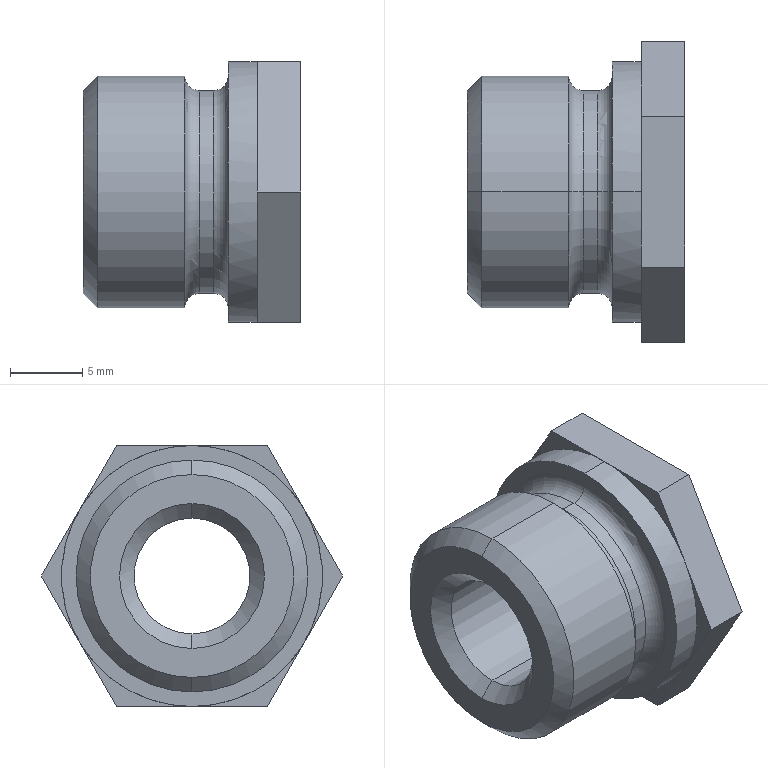Part | SolidWorks | features BaseBody 1 | 1 solid | 33 faces | box 15 x 20.785 x 18 mm | volume 2434 mm3 | plane 15 | cylinder 8 | cone 6 | torus 4 | commonest cylinder face diameters 8 x2 14 x2 16 x2 18 x2
STEP:
#1=CARTESIAN_POINT('',(-9.463,-20.104,-29.75));
#2=VERTEX_POINT('',#1);
#3=CARTESIAN_POINT('',(-9.463,-20.104,-47.75));
#4=VERTEX_POINT('',#3);
#5=CARTESIAN_POINT('',(-9.463,-20.104,-38.75));
#6=DIRECTION('',(-1.,0.,0.));
#7=DIRECTION('',(0.,0.,1.));
#8=AXIS2_PLACEMENT_3D('',#5,#6,#7);
#9=CIRCLE('',#8,9.);
#10=EDGE_CURVE('',#2,#4,#9,.T.);
#11=ORIENTED_EDGE('',*,*,#10,.F.);
#12=CARTESIAN_POINT('',(-7.463,-20.104,-29.75));
#13=VERTEX_POINT('',#12);
#14=CARTESIAN_POINT('',(-9.463,-20.104,-29.75));
#15=DIRECTION('',(1.,0.,0.));
#16=VECTOR('',#15,1000.);
#17=LINE('',#14,#16);
#18=EDGE_CURVE('',#2,#13,#17,.T.);
#19=ORIENTED_EDGE('',*,*,#18,.T.);
#20=CARTESIAN_POINT('',(-7.463,-12.31,-34.25));
#21=VERTEX_POINT('',#20);
#22=CARTESIAN_POINT('',(-7.463,-20.104,-38.75));
#23=DIRECTION('',(-1.,0.,0.));
#24=DIRECTION('',(0.,0.,1.));
#25=AXIS2_PLACEMENT_3D('',#22,#23,#24);
#26=CIRCLE('',#25,9.);
#27=EDGE_CURVE('',#13,#21,#26,.T.);
#28=ORIENTED_EDGE('',*,*,#27,.T.);
#29=CARTESIAN_POINT('',(-7.463,-12.31,-43.25));
#30=VERTEX_POINT('',#29);
#31=CARTESIAN_POINT('',(-7.463,-20.104,-38.75));
#32=DIRECTION('',(-1.,0.,0.));
#33=DIRECTION('',(0.,0.,1.));
#34=AXIS2_PLACEMENT_3D('',#31,#32,#33);
#35=CIRCLE('',#34,9.);
#36=EDGE_CURVE('',#21,#30,#35,.T.);
#37=ORIENTED_EDGE('',*,*,#36,.T.);
#38=CARTESIAN_POINT('',(-7.463,-20.104,-47.75));
#39=VERTEX_POINT('',#38);
#40=CARTESIAN_POINT('',(-7.463,-20.104,-38.75));
#41=DIRECTION('',(-1.,0.,0.));
#42=DIRECTION('',(0.,0.,1.));
#43=AXIS2_PLACEMENT_3D('',#40,#41,#42);
#44=CIRCLE('',#43,9.);
#45=EDGE_CURVE('',#30,#39,#44,.T.);
#46=ORIENTED_EDGE('',*,*,#45,.T.);
#47=CARTESIAN_POINT('',(-9.463,-20.104,-47.75));
#48=DIRECTION('',(1.,0.,0.));
#49=VECTOR('',#48,1000.);
#50=LINE('',#47,#49);
#51=EDGE_CURVE('',#4,#39,#50,.T.);
#52=ORIENTED_EDGE('',*,*,#51,.F.);
#53=EDGE_LOOP('',(#11,#19,#28,#37,#46,#52));
#54=FACE_OUTER_BOUND('',#53,.T.);
#55=CARTESIAN_POINT('',(-9.463,-20.104,-38.75));
#56=DIRECTION('',(1.,0.,0.));
#57=DIRECTION('',(0.,0.,-1.));
#58=AXIS2_PLACEMENT_3D('',#55,#56,#57);
#59=CYLINDRICAL_SURFACE('',#58,9.);
#60=ADVANCED_FACE('',(#54),#59,.T.);
#61=CARTESIAN_POINT('',(-11.463,-20.104,-45.75));
#62=VERTEX_POINT('',#61);
#63=CARTESIAN_POINT('',(-11.463,-20.104,-31.75));
#64=VERTEX_POINT('',#63);
#65=CARTESIAN_POINT('',(-11.463,-20.104,-38.75));
#66=DIRECTION('',(1.,0.,0.));
#67=DIRECTION('',(0.,0.,1.));
#68=AXIS2_PLACEMENT_3D('',#65,#66,#67);
#69=CIRCLE('',#68,7.);
#70=EDGE_CURVE('',#62,#64,#69,.T.);
#71=ORIENTED_EDGE('',*,*,#70,.T.);
#72=CARTESIAN_POINT('',(-10.463,-20.104,-31.75));
#73=VERTEX_POINT('',#72);
#74=CARTESIAN_POINT('',(-12.463,-20.104,-31.75));
#75=DIRECTION('',(1.,0.,0.));
#76=VECTOR('',#75,1000.);
#77=LINE('',#74,#76);
#78=EDGE_CURVE('',#64,#73,#77,.T.);
#79=ORIENTED_EDGE('',*,*,#78,.T.);
#80=CARTESIAN_POINT('',(-10.463,-20.104,-45.75));
#81=VERTEX_POINT('',#80);
#82=CARTESIAN_POINT('',(-10.463,-20.104,-38.75));
#83=DIRECTION('',(-1.,0.,0.));
#84=DIRECTION('',(0.,0.,1.));
#85=AXIS2_PLACEMENT_3D('',#82,#83,#84);
#86=CIRCLE('',#85,7.);
#87=EDGE_CURVE('',#73,#81,#86,.T.);
#88=ORIENTED_EDGE('',*,*,#87,.T.);
#89=CARTESIAN_POINT('',(-12.463,-20.104,-45.75));
#90=DIRECTION('',(1.,0.,0.));
#91=VECTOR('',#90,1000.);
#92=LINE('',#89,#91);
#93=EDGE_CURVE('',#62,#81,#92,.T.);
#94=ORIENTED_EDGE('',*,*,#93,.F.);
#95=EDGE_LOOP('',(#71,#79,#88,#94));
#96=FACE_OUTER_BOUND('',#95,.T.);
#97=CARTESIAN_POINT('',(-12.463,-20.104,-38.75));
#98=DIRECTION('',(1.,0.,0.));
#99=DIRECTION('',(0.,0.,-1.));
#100=AXIS2_PLACEMENT_3D('',#97,#98,#99);
#101=CYLINDRICAL_SURFACE('',#100,7.);
#102=ADVANCED_FACE('',(#96),#101,.T.);
#103=CARTESIAN_POINT('',(-18.463,-20.104,-46.75));
#104=VERTEX_POINT('',#103);
#105=CARTESIAN_POINT('',(-18.463,-20.104,-30.75));
#106=VERTEX_POINT('',#105);
#107=CARTESIAN_POINT('',(-18.463,-20.104,-38.75));
#108=DIRECTION('',(1.,0.,0.));
#109=DIRECTION('',(0.,0.,1.));
#110=AXIS2_PLACEMENT_3D('',#107,#108,#109);
#111=CIRCLE('',#110,8.);
#112=EDGE_CURVE('',#104,#106,#111,.T.);
#113=ORIENTED_EDGE('',*,*,#112,.T.);
#114=CARTESIAN_POINT('',(-12.463,-20.104,-30.75));
#115=VERTEX_POINT('',#114);
#116=CARTESIAN_POINT('',(-19.463,-20.104,-30.75));
#117=DIRECTION('',(1.,0.,0.));
#118=VECTOR('',#117,1000.);
#119=LINE('',#116,#118);
#120=EDGE_CURVE('',#106,#115,#119,.T.);
#121=ORIENTED_EDGE('',*,*,#120,.T.);
#122=CARTESIAN_POINT('',(-12.463,-20.104,-46.75));
#123=VERTEX_POINT('',#122);
#124=CARTESIAN_POINT('',(-12.463,-20.104,-38.75));
#125=DIRECTION('',(-1.,0.,0.));
#126=DIRECTION('',(0.,0.,1.));
#127=AXIS2_PLACEMENT_3D('',#124,#125,#126);
#128=CIRCLE('',#127,8.);
#129=EDGE_CURVE('',#115,#123,#128,.T.);
#130=ORIENTED_EDGE('',*,*,#129,.T.);
#131=CARTESIAN_POINT('',(-19.463,-20.104,-46.75));
#132=DIRECTION('',(1.,0.,0.));
#133=VECTOR('',#132,1000.);
#134=LINE('',#131,#133);
#135=EDGE_CURVE('',#104,#123,#134,.T.);
#136=ORIENTED_EDGE('',*,*,#135,.F.);
#137=EDGE_LOOP('',(#113,#121,#130,#136));
#138=FACE_OUTER_BOUND('',#137,.T.);
#139=CARTESIAN_POINT('',(-19.463,-20.104,-38.75));
#140=DIRECTION('',(1.,0.,0.));
#141=DIRECTION('',(0.,0.,-1.));
#142=AXIS2_PLACEMENT_3D('',#139,#140,#141);
#143=CYLINDRICAL_SURFACE('',#142,8.);
#144=ADVANCED_FACE('',(#138),#143,.T.);
#145=CARTESIAN_POINT('',(-10.463,-20.104,-38.75));
#146=DIRECTION('',(-1.,0.,0.));
#147=DIRECTION('',(0.,0.,1.));
#148=AXIS2_PLACEMENT_3D('',#145,#146,#147);
#149=CIRCLE('',#148,7.);
#150=EDGE_CURVE('',#81,#73,#149,.T.);
#151=ORIENTED_EDGE('',*,*,#150,.F.);
#152=CARTESIAN_POINT('',(-9.463,-20.104,-46.75));
#153=VERTEX_POINT('',#152);
#154=CARTESIAN_POINT('',(-10.463,-20.104,-46.75));
#155=DIRECTION('',(0.,1.,0.));
#156=DIRECTION('',(0.,0.,1.));
#157=AXIS2_PLACEMENT_3D('',#154,#155,#156);
#158=CIRCLE('',#157,1.);
#159=EDGE_CURVE('',#81,#153,#158,.T.);
#160=ORIENTED_EDGE('',*,*,#159,.T.);
#161=CARTESIAN_POINT('',(-9.463,-20.104,-30.75));
#162=VERTEX_POINT('',#161);
#163=CARTESIAN_POINT('',(-9.463,-20.104,-38.75));
#164=DIRECTION('',(1.,0.,0.));
#165=DIRECTION('',(0.,0.,1.));
#166=AXIS2_PLACEMENT_3D('',#163,#164,#165);
#167=CIRCLE('',#166,8.);
#168=EDGE_CURVE('',#162,#153,#167,.T.);
#169=ORIENTED_EDGE('',*,*,#168,.F.);
#170=CARTESIAN_POINT('',(-10.463,-20.104,-30.75));
#171=DIRECTION('',(0.,-1.,0.));
#172=DIRECTION('',(0.,0.,-1.));
#173=AXIS2_PLACEMENT_3D('',#170,#171,#172);
#174=CIRCLE('',#173,1.);
#175=EDGE_CURVE('',#73,#162,#174,.T.);
#176=ORIENTED_EDGE('',*,*,#175,.F.);
#177=EDGE_LOOP('',(#151,#160,#169,#176));
#178=FACE_OUTER_BOUND('',#177,.T.);
#179=CARTESIAN_POINT('',(-10.463,-20.104,-38.75));
#180=DIRECTION('',(-1.,0.,0.));
#181=DIRECTION('',(0.,0.,1.));
#182=AXIS2_PLACEMENT_3D('',#179,#180,#181);
#183=TOROIDAL_SURFACE('',#182,8.,1.);
#184=ADVANCED_FACE('',(#178),#183,.F.);
#185=CARTESIAN_POINT('',(-12.463,-20.104,-38.75));
#186=DIRECTION('',(-1.,0.,0.));
#187=DIRECTION('',(0.,0.,1.));
#188=AXIS2_PLACEMENT_3D('',#185,#186,#187);
#189=CIRCLE('',#188,8.);
#190=EDGE_CURVE('',#123,#115,#189,.T.);
#191=ORIENTED_EDGE('',*,*,#190,.F.);
#192=CARTESIAN_POINT('',(-11.463,-20.104,-46.75));
#193=DIRECTION('',(0.,1.,0.));
#194=DIRECTION('',(0.,0.,1.));
#195=AXIS2_PLACEMENT_3D('',#192,#193,#194);
#196=CIRCLE('',#195,1.);
#197=EDGE_CURVE('',#123,#62,#196,.T.);
#198=ORIENTED_EDGE('',*,*,#197,.T.);
#199=CARTESIAN_POINT('',(-11.463,-20.104,-38.75));
#200=DIRECTION('',(1.,0.,0.));
#201=DIRECTION('',(0.,0.,1.));
#202=AXIS2_PLACEMENT_3D('',#199,#200,#201);
#203=CIRCLE('',#202,7.);
#204=EDGE_CURVE('',#64,#62,#203,.T.);
#205=ORIENTED_EDGE('',*,*,#204,.F.);
#206=CARTESIAN_POINT('',(-11.463,-20.104,-30.75));
#207=DIRECTION('',(0.,-1.,0.));
#208=DIRECTION('',(0.,0.,-1.));
#209=AXIS2_PLACEMENT_3D('',#206,#207,#208);
#210=CIRCLE('',#209,1.);
#211=EDGE_CURVE('',#115,#64,#210,.T.);
#212=ORIENTED_EDGE('',*,*,#211,.F.);
#213=EDGE_LOOP('',(#191,#198,#205,#212));
#214=FACE_OUTER_BOUND('',#213,.T.);
#215=CARTESIAN_POINT('',(-11.463,-20.104,-38.75));
#216=DIRECTION('',(-1.,0.,0.));
#217=DIRECTION('',(0.,0.,1.));
#218=AXIS2_PLACEMENT_3D('',#215,#216,#217);
#219=TOROIDAL_SURFACE('',#218,8.,1.);
#220=ADVANCED_FACE('',(#214),#219,.F.);
#221=CARTESIAN_POINT('',(-19.463,-20.104,-31.75));
#222=VERTEX_POINT('',#221);
#223=CARTESIAN_POINT('',(-19.463,-20.104,-45.75));
#224=VERTEX_POINT('',#223);
#225=CARTESIAN_POINT('',(-19.463,-20.104,-38.75));
#226=DIRECTION('',(-1.,0.,0.));
#227=DIRECTION('',(0.,0.,1.));
#228=AXIS2_PLACEMENT_3D('',#225,#226,#227);
#229=CIRCLE('',#228,7.);
#230=EDGE_CURVE('',#222,#224,#229,.T.);
#231=ORIENTED_EDGE('',*,*,#230,.F.);
#232=CARTESIAN_POINT('',(-19.463,-20.104,-31.75));
#233=DIRECTION('',(0.7071,0.,0.7071));
#234=VECTOR('',#233,1000.);
#235=LINE('',#232,#234);
#236=EDGE_CURVE('',#222,#106,#235,.T.);
#237=ORIENTED_EDGE('',*,*,#236,.T.);
#238=ORIENTED_EDGE('',*,*,#112,.F.);
#239=CARTESIAN_POINT('',(-19.463,-20.104,-45.75));
#240=DIRECTION('',(0.7071,0.,-0.7071));
#241=VECTOR('',#240,1000.);
#242=LINE('',#239,#241);
#243=EDGE_CURVE('',#224,#104,#242,.T.);
#244=ORIENTED_EDGE('',*,*,#243,.F.);
#245=EDGE_LOOP('',(#231,#237,#238,#244));
#246=FACE_OUTER_BOUND('',#245,.T.);
#247=CARTESIAN_POINT('',(-19.463,-20.104,-38.75));
#248=DIRECTION('',(1.,0.,0.));
#249=DIRECTION('',(0.,0.,-1.));
#250=AXIS2_PLACEMENT_3D('',#247,#248,#249);
#251=CONICAL_SURFACE('',#250,7.,0.7854);
#252=ADVANCED_FACE('',(#246),#251,.T.);
#253=CARTESIAN_POINT('',(-5.463,-20.104,-34.75));
#254=VERTEX_POINT('',#253);
#255=CARTESIAN_POINT('',(-5.463,-20.104,-42.75));
#256=VERTEX_POINT('',#255);
#257=CARTESIAN_POINT('',(-5.463,-20.104,-38.75));
#258=DIRECTION('',(1.,0.,0.));
#259=DIRECTION('',(0.,0.,1.));
#260=AXIS2_PLACEMENT_3D('',#257,#258,#259);
#261=CIRCLE('',#260,4.);
#262=EDGE_CURVE('',#254,#256,#261,.T.);
#263=ORIENTED_EDGE('',*,*,#262,.T.);
#264=CARTESIAN_POINT('',(-18.463,-20.104,-42.75));
#265=VERTEX_POINT('',#264);
#266=CARTESIAN_POINT('',(-4.463,-20.104,-42.75));
#267=DIRECTION('',(-1.,0.,0.));
#268=VECTOR('',#267,1000.);
#269=LINE('',#266,#268);
#270=EDGE_CURVE('',#256,#265,#269,.T.);
#271=ORIENTED_EDGE('',*,*,#270,.T.);
#272=CARTESIAN_POINT('',(-18.463,-20.104,-34.75));
#273=VERTEX_POINT('',#272);
#274=CARTESIAN_POINT('',(-18.463,-20.104,-38.75));
#275=DIRECTION('',(-1.,0.,0.));
#276=DIRECTION('',(0.,0.,1.));
#277=AXIS2_PLACEMENT_3D('',#274,#275,#276);
#278=CIRCLE('',#277,4.);
#279=EDGE_CURVE('',#265,#273,#278,.T.);
#280=ORIENTED_EDGE('',*,*,#279,.T.);
#281=CARTESIAN_POINT('',(-4.463,-20.104,-34.75));
#282=DIRECTION('',(-1.,0.,0.));
#283=VECTOR('',#282,1000.);
#284=LINE('',#281,#283);
#285=EDGE_CURVE('',#254,#273,#284,.T.);
#286=ORIENTED_EDGE('',*,*,#285,.F.);
#287=EDGE_LOOP('',(#263,#271,#280,#286));
#288=FACE_OUTER_BOUND('',#287,.T.);
#289=CARTESIAN_POINT('',(-4.463,-20.104,-38.75));
#290=DIRECTION('',(-1.,0.,0.));
#291=DIRECTION('',(0.,0.,1.));
#292=AXIS2_PLACEMENT_3D('',#289,#290,#291);
#293=CYLINDRICAL_SURFACE('',#292,4.);
#294=ADVANCED_FACE('',(#288),#293,.F.);
#295=ORIENTED_EDGE('',*,*,#279,.F.);
#296=CARTESIAN_POINT('',(-19.463,-20.104,-43.75));
#297=VERTEX_POINT('',#296);
#298=CARTESIAN_POINT('',(-18.463,-20.104,-42.75));
#299=DIRECTION('',(-0.7071,0.,-0.7071));
#300=VECTOR('',#299,1000.);
#301=LINE('',#298,#300);
#302=EDGE_CURVE('',#265,#297,#301,.T.);
#303=ORIENTED_EDGE('',*,*,#302,.T.);
#304=CARTESIAN_POINT('',(-19.463,-20.104,-33.75));
#305=VERTEX_POINT('',#304);
#306=CARTESIAN_POINT('',(-19.463,-20.104,-38.75));
#307=DIRECTION('',(1.,0.,0.));
#308=DIRECTION('',(0.,0.,1.));
#309=AXIS2_PLACEMENT_3D('',#306,#307,#308);
#310=CIRCLE('',#309,5.);
#311=EDGE_CURVE('',#305,#297,#310,.T.);
#312=ORIENTED_EDGE('',*,*,#311,.F.);
#313=CARTESIAN_POINT('',(-18.463,-20.104,-34.75));
#314=DIRECTION('',(-0.7071,0.,0.7071));
#315=VECTOR('',#314,1000.);
#316=LINE('',#313,#315);
#317=EDGE_CURVE('',#273,#305,#316,.T.);
#318=ORIENTED_EDGE('',*,*,#317,.F.);
#319=EDGE_LOOP('',(#295,#303,#312,#318));
#320=FACE_OUTER_BOUND('',#319,.T.);
#321=CARTESIAN_POINT('',(-18.463,-20.104,-38.75));
#322=DIRECTION('',(-1.,0.,0.));
#323=DIRECTION('',(0.,0.,1.));
#324=AXIS2_PLACEMENT_3D('',#321,#322,#323);
#325=CONICAL_SURFACE('',#324,4.,0.7854);
#326=ADVANCED_FACE('',(#320),#325,.F.);
#327=ORIENTED_EDGE('',*,*,#262,.F.);
#328=CARTESIAN_POINT('',(-4.463,-20.104,-33.75));
#329=VERTEX_POINT('',#328);
#330=CARTESIAN_POINT('',(-4.463,-20.104,-33.75));
#331=DIRECTION('',(0.7071,0.,0.7071));
#332=VECTOR('',#331,1000.);
#333=LINE('',#330,#332);
#334=EDGE_CURVE('',#254,#329,#333,.T.);
#335=ORIENTED_EDGE('',*,*,#334,.T.);
#336=CARTESIAN_POINT('',(-4.463,-20.104,-43.75));
#337=VERTEX_POINT('',#336);
#338=CARTESIAN_POINT('',(-4.463,-20.104,-38.75));
#339=DIRECTION('',(-1.,0.,0.));
#340=DIRECTION('',(0.,0.,1.));
#341=AXIS2_PLACEMENT_3D('',#338,#339,#340);
#342=CIRCLE('',#341,5.);
#343=EDGE_CURVE('',#337,#329,#342,.T.);
#344=ORIENTED_EDGE('',*,*,#343,.F.);
#345=CARTESIAN_POINT('',(-4.463,-20.104,-43.75));
#346=DIRECTION('',(0.7071,0.,-0.7071));
#347=VECTOR('',#346,1000.);
#348=LINE('',#345,#347);
#349=EDGE_CURVE('',#256,#337,#348,.T.);
#350=ORIENTED_EDGE('',*,*,#349,.F.);
#351=EDGE_LOOP('',(#327,#335,#344,#350));
#352=FACE_OUTER_BOUND('',#351,.T.);
#353=CARTESIAN_POINT('',(-4.463,-20.104,-38.75));
#354=DIRECTION('',(1.,0.,0.));
#355=DIRECTION('',(0.,0.,-1.));
#356=AXIS2_PLACEMENT_3D('',#353,#354,#355);
#357=CONICAL_SURFACE('',#356,5.,0.7854);
#358=ADVANCED_FACE('',(#352),#357,.F.);
#359=ORIENTED_EDGE('',*,*,#334,.F.);
#360=CARTESIAN_POINT('',(-5.463,-20.104,-38.75));
#361=DIRECTION('',(1.,0.,0.));
#362=DIRECTION('',(0.,0.,1.));
#363=AXIS2_PLACEMENT_3D('',#360,#361,#362);
#364=CIRCLE('',#363,4.);
#365=EDGE_CURVE('',#256,#254,#364,.T.);
#366=ORIENTED_EDGE('',*,*,#365,.F.);
#367=ORIENTED_EDGE('',*,*,#349,.T.);
#368=CARTESIAN_POINT('',(-4.463,-20.104,-38.75));
#369=DIRECTION('',(-1.,0.,0.));
#370=DIRECTION('',(0.,0.,1.));
#371=AXIS2_PLACEMENT_3D('',#368,#369,#370);
#372=CIRCLE('',#371,5.);
#373=EDGE_CURVE('',#329,#337,#372,.T.);
#374=ORIENTED_EDGE('',*,*,#373,.F.);
#375=EDGE_LOOP('',(#359,#366,#367,#374));
#376=FACE_OUTER_BOUND('',#375,.T.);
#377=CARTESIAN_POINT('',(-4.463,-20.104,-38.75));
#378=DIRECTION('',(1.,0.,0.));
#379=DIRECTION('',(0.,0.,-1.));
#380=AXIS2_PLACEMENT_3D('',#377,#378,#379);
#381=CONICAL_SURFACE('',#380,5.,0.7854);
#382=ADVANCED_FACE('',(#376),#381,.F.);
#383=ORIENTED_EDGE('',*,*,#302,.F.);
#384=CARTESIAN_POINT('',(-18.463,-20.104,-38.75));
#385=DIRECTION('',(-1.,0.,0.));
#386=DIRECTION('',(0.,0.,1.));
#387=AXIS2_PLACEMENT_3D('',#384,#385,#386);
#388=CIRCLE('',#387,4.);
#389=EDGE_CURVE('',#273,#265,#388,.T.);
#390=ORIENTED_EDGE('',*,*,#389,.F.);
#391=ORIENTED_EDGE('',*,*,#317,.T.);
#392=CARTESIAN_POINT('',(-19.463,-20.104,-38.75));
#393=DIRECTION('',(1.,0.,0.));
#394=DIRECTION('',(0.,0.,1.));
#395=AXIS2_PLACEMENT_3D('',#392,#393,#394);
#396=CIRCLE('',#395,5.);
#397=EDGE_CURVE('',#297,#305,#396,.T.);
#398=ORIENTED_EDGE('',*,*,#397,.F.);
#399=EDGE_LOOP('',(#383,#390,#391,#398));
#400=FACE_OUTER_BOUND('',#399,.T.);
#401=CARTESIAN_POINT('',(-18.463,-20.104,-38.75));
#402=DIRECTION('',(-1.,0.,0.));
#403=DIRECTION('',(0.,0.,1.));
#404=AXIS2_PLACEMENT_3D('',#401,#402,#403);
#405=CONICAL_SURFACE('',#404,4.,0.7854);
#406=ADVANCED_FACE('',(#400),#405,.F.);
#407=ORIENTED_EDGE('',*,*,#270,.F.);
#408=ORIENTED_EDGE('',*,*,#365,.T.);
#409=ORIENTED_EDGE('',*,*,#285,.T.);
#410=ORIENTED_EDGE('',*,*,#389,.T.);
#411=EDGE_LOOP('',(#407,#408,#409,#410));
#412=FACE_OUTER_BOUND('',#411,.T.);
#413=CARTESIAN_POINT('',(-4.463,-20.104,-38.75));
#414=DIRECTION('',(-1.,0.,0.));
#415=DIRECTION('',(0.,0.,1.));
#416=AXIS2_PLACEMENT_3D('',#413,#414,#415);
#417=CYLINDRICAL_SURFACE('',#416,4.);
#418=ADVANCED_FACE('',(#412),#417,.F.);
#419=ORIENTED_EDGE('',*,*,#236,.F.);
#420=CARTESIAN_POINT('',(-19.463,-20.104,-38.75));
#421=DIRECTION('',(-1.,0.,0.));
#422=DIRECTION('',(0.,0.,1.));
#423=AXIS2_PLACEMENT_3D('',#420,#421,#422);
#424=CIRCLE('',#423,7.);
#425=EDGE_CURVE('',#224,#222,#424,.T.);
#426=ORIENTED_EDGE('',*,*,#425,.F.);
#427=ORIENTED_EDGE('',*,*,#243,.T.);
#428=CARTESIAN_POINT('',(-18.463,-20.104,-38.75));
#429=DIRECTION('',(1.,0.,0.));
#430=DIRECTION('',(0.,0.,1.));
#431=AXIS2_PLACEMENT_3D('',#428,#429,#430);
#432=CIRCLE('',#431,8.);
#433=EDGE_CURVE('',#106,#104,#432,.T.);
#434=ORIENTED_EDGE('',*,*,#433,.F.);
#435=EDGE_LOOP('',(#419,#426,#427,#434));
#436=FACE_OUTER_BOUND('',#435,.T.);
#437=CARTESIAN_POINT('',(-19.463,-20.104,-38.75));
#438=DIRECTION('',(1.,0.,0.));
#439=DIRECTION('',(0.,0.,-1.));
#440=AXIS2_PLACEMENT_3D('',#437,#438,#439);
#441=CONICAL_SURFACE('',#440,7.,0.7854);
#442=ADVANCED_FACE('',(#436),#441,.T.);
#443=ORIENTED_EDGE('',*,*,#197,.F.);
#444=ORIENTED_EDGE('',*,*,#129,.F.);
#445=ORIENTED_EDGE('',*,*,#211,.T.);
#446=ORIENTED_EDGE('',*,*,#70,.F.);
#447=EDGE_LOOP('',(#443,#444,#445,#446));
#448=FACE_OUTER_BOUND('',#447,.T.);
#449=CARTESIAN_POINT('',(-11.463,-20.104,-38.75));
#450=DIRECTION('',(-1.,0.,0.));
#451=DIRECTION('',(0.,0.,1.));
#452=AXIS2_PLACEMENT_3D('',#449,#450,#451);
#453=TOROIDAL_SURFACE('',#452,8.,1.);
#454=ADVANCED_FACE('',(#448),#453,.F.);
#455=ORIENTED_EDGE('',*,*,#159,.F.);
#456=ORIENTED_EDGE('',*,*,#87,.F.);
#457=ORIENTED_EDGE('',*,*,#175,.T.);
#458=CARTESIAN_POINT('',(-9.463,-20.104,-38.75));
#459=DIRECTION('',(1.,0.,0.));
#460=DIRECTION('',(0.,0.,1.));
#461=AXIS2_PLACEMENT_3D('',#458,#459,#460);
#462=CIRCLE('',#461,8.);
#463=EDGE_CURVE('',#153,#162,#462,.T.);
#464=ORIENTED_EDGE('',*,*,#463,.F.);
#465=EDGE_LOOP('',(#455,#456,#457,#464));
#466=FACE_OUTER_BOUND('',#465,.T.);
#467=CARTESIAN_POINT('',(-10.463,-20.104,-38.75));
#468=DIRECTION('',(-1.,0.,0.));
#469=DIRECTION('',(0.,0.,1.));
#470=AXIS2_PLACEMENT_3D('',#467,#468,#469);
#471=TOROIDAL_SURFACE('',#470,8.,1.);
#472=ADVANCED_FACE('',(#466),#471,.F.);
#473=ORIENTED_EDGE('',*,*,#425,.T.);
#474=ORIENTED_EDGE('',*,*,#230,.T.);
#475=EDGE_LOOP('',(#473,#474));
#476=FACE_OUTER_BOUND('',#475,.T.);
#477=ORIENTED_EDGE('',*,*,#311,.T.);
#478=ORIENTED_EDGE('',*,*,#397,.T.);
#479=EDGE_LOOP('',(#477,#478));
#480=FACE_BOUND('',#479,.T.);
#481=CARTESIAN_POINT('',(-19.463,-20.104,-38.75));
#482=DIRECTION('',(-1.,0.,0.));
#483=DIRECTION('',(0.,1.,0.));
#484=AXIS2_PLACEMENT_3D('',#481,#482,#483);
#485=PLANE('',#484);
#486=ADVANCED_FACE('',(#476,#480),#485,.T.);
#487=ORIENTED_EDGE('',*,*,#120,.F.);
#488=ORIENTED_EDGE('',*,*,#433,.T.);
#489=ORIENTED_EDGE('',*,*,#135,.T.);
#490=ORIENTED_EDGE('',*,*,#190,.T.);
#491=EDGE_LOOP('',(#487,#488,#489,#490));
#492=FACE_OUTER_BOUND('',#491,.T.);
#493=CARTESIAN_POINT('',(-19.463,-20.104,-38.75));
#494=DIRECTION('',(1.,0.,0.));
#495=DIRECTION('',(0.,0.,-1.));
#496=AXIS2_PLACEMENT_3D('',#493,#494,#495);
#497=CYLINDRICAL_SURFACE('',#496,8.);
#498=ADVANCED_FACE('',(#492),#497,.T.);
#499=ORIENTED_EDGE('',*,*,#78,.F.);
#500=ORIENTED_EDGE('',*,*,#204,.T.);
#501=ORIENTED_EDGE('',*,*,#93,.T.);
#502=ORIENTED_EDGE('',*,*,#150,.T.);
#503=EDGE_LOOP('',(#499,#500,#501,#502));
#504=FACE_OUTER_BOUND('',#503,.T.);
#505=CARTESIAN_POINT('',(-12.463,-20.104,-38.75));
#506=DIRECTION('',(1.,0.,0.));
#507=DIRECTION('',(0.,0.,-1.));
#508=AXIS2_PLACEMENT_3D('',#505,#506,#507);
#509=CYLINDRICAL_SURFACE('',#508,7.);
#510=ADVANCED_FACE('',(#504),#509,.T.);
#511=ORIENTED_EDGE('',*,*,#18,.F.);
#512=CARTESIAN_POINT('',(-9.463,-20.104,-38.75));
#513=DIRECTION('',(-1.,0.,0.));
#514=DIRECTION('',(0.,0.,1.));
#515=AXIS2_PLACEMENT_3D('',#512,#513,#514);
#516=CIRCLE('',#515,9.);
#517=EDGE_CURVE('',#4,#2,#516,.T.);
#518=ORIENTED_EDGE('',*,*,#517,.F.);
#519=ORIENTED_EDGE('',*,*,#51,.T.);
#520=CARTESIAN_POINT('',(-7.463,-27.898,-43.25));
#521=VERTEX_POINT('',#520);
#522=CARTESIAN_POINT('',(-7.463,-20.104,-38.75));
#523=DIRECTION('',(-1.,0.,0.));
#524=DIRECTION('',(0.,0.,1.));
#525=AXIS2_PLACEMENT_3D('',#522,#523,#524);
#526=CIRCLE('',#525,9.);
#527=EDGE_CURVE('',#39,#521,#526,.T.);
#528=ORIENTED_EDGE('',*,*,#527,.T.);
#529=CARTESIAN_POINT('',(-7.463,-27.898,-34.25));
#530=VERTEX_POINT('',#529);
#531=CARTESIAN_POINT('',(-7.463,-20.104,-38.75));
#532=DIRECTION('',(-1.,0.,0.));
#533=DIRECTION('',(0.,0.,1.));
#534=AXIS2_PLACEMENT_3D('',#531,#532,#533);
#535=CIRCLE('',#534,9.);
#536=EDGE_CURVE('',#521,#530,#535,.T.);
#537=ORIENTED_EDGE('',*,*,#536,.T.);
#538=CARTESIAN_POINT('',(-7.463,-20.104,-38.75));
#539=DIRECTION('',(-1.,0.,0.));
#540=DIRECTION('',(0.,0.,1.));
#541=AXIS2_PLACEMENT_3D('',#538,#539,#540);
#542=CIRCLE('',#541,9.);
#543=EDGE_CURVE('',#530,#13,#542,.T.);
#544=ORIENTED_EDGE('',*,*,#543,.T.);
#545=EDGE_LOOP('',(#511,#518,#519,#528,#537,#544));
#546=FACE_OUTER_BOUND('',#545,.T.);
#547=CARTESIAN_POINT('',(-9.463,-20.104,-38.75));
#548=DIRECTION('',(1.,0.,0.));
#549=DIRECTION('',(0.,0.,-1.));
#550=AXIS2_PLACEMENT_3D('',#547,#548,#549);
#551=CYLINDRICAL_SURFACE('',#550,9.);
#552=ADVANCED_FACE('',(#546),#551,.T.);
#553=CARTESIAN_POINT('',(-4.463,-9.711,-38.75));
#554=VERTEX_POINT('',#553);
#555=CARTESIAN_POINT('',(-4.463,-14.908,-47.75));
#556=VERTEX_POINT('',#555);
#557=CARTESIAN_POINT('',(-4.463,-9.711,-38.75));
#558=DIRECTION('',(0.,-0.5,-0.866));
#559=VECTOR('',#558,1000.);
#560=LINE('',#557,#559);
#561=EDGE_CURVE('',#554,#556,#560,.T.);
#562=ORIENTED_EDGE('',*,*,#561,.F.);
#563=CARTESIAN_POINT('',(-4.463,-14.908,-29.75));
#564=VERTEX_POINT('',#563);
#565=CARTESIAN_POINT('',(-4.463,-9.711,-38.75));
#566=DIRECTION('',(0.,0.5,-0.866));
#567=VECTOR('',#566,1000.);
#568=LINE('',#565,#567);
#569=EDGE_CURVE('',#564,#554,#568,.T.);
#570=ORIENTED_EDGE('',*,*,#569,.F.);
#571=CARTESIAN_POINT('',(-4.463,-25.3,-29.75));
#572=VERTEX_POINT('',#571);
#573=CARTESIAN_POINT('',(-4.463,-14.908,-29.75));
#574=DIRECTION('',(0.,1.,0.));
#575=VECTOR('',#574,1000.);
#576=LINE('',#573,#575);
#577=EDGE_CURVE('',#572,#564,#576,.T.);
#578=ORIENTED_EDGE('',*,*,#577,.F.);
#579=CARTESIAN_POINT('',(-4.463,-30.496,-38.75));
#580=VERTEX_POINT('',#579);
#581=CARTESIAN_POINT('',(-4.463,-25.3,-29.75));
#582=DIRECTION('',(0.,0.5,0.866));
#583=VECTOR('',#582,1000.);
#584=LINE('',#581,#583);
#585=EDGE_CURVE('',#580,#572,#584,.T.);
#586=ORIENTED_EDGE('',*,*,#585,.F.);
#587=CARTESIAN_POINT('',(-4.463,-25.3,-47.75));
#588=VERTEX_POINT('',#587);
#589=CARTESIAN_POINT('',(-4.463,-25.3,-47.75));
#590=DIRECTION('',(0.,-0.5,0.866));
#591=VECTOR('',#590,1000.);
#592=LINE('',#589,#591);
#593=EDGE_CURVE('',#588,#580,#592,.T.);
#594=ORIENTED_EDGE('',*,*,#593,.F.);
#595=CARTESIAN_POINT('',(-4.463,-14.908,-47.75));
#596=DIRECTION('',(0.,-1.,0.));
#597=VECTOR('',#596,1000.);
#598=LINE('',#595,#597);
#599=EDGE_CURVE('',#556,#588,#598,.T.);
#600=ORIENTED_EDGE('',*,*,#599,.F.);
#601=EDGE_LOOP('',(#562,#570,#578,#586,#594,#600));
#602=FACE_OUTER_BOUND('',#601,.T.);
#603=ORIENTED_EDGE('',*,*,#343,.T.);
#604=ORIENTED_EDGE('',*,*,#373,.T.);
#605=EDGE_LOOP('',(#603,#604));
#606=FACE_BOUND('',#605,.T.);
#607=CARTESIAN_POINT('',(-4.463,-20.104,-56.75));
#608=DIRECTION('',(-1.,0.,0.));
#609=DIRECTION('',(0.,1.,0.));
#610=AXIS2_PLACEMENT_3D('',#607,#608,#609);
#611=PLANE('',#610);
#612=ADVANCED_FACE('',(#602,#606),#611,.F.);
#613=ORIENTED_EDGE('',*,*,#543,.F.);
#614=CARTESIAN_POINT('',(-7.463,-25.3,-29.75));
#615=VERTEX_POINT('',#614);
#616=CARTESIAN_POINT('',(-7.463,-25.3,-29.75));
#617=DIRECTION('',(0.,0.5,0.866));
#618=VECTOR('',#617,1000.);
#619=LINE('',#616,#618);
#620=EDGE_CURVE('',#530,#615,#619,.T.);
#621=ORIENTED_EDGE('',*,*,#620,.T.);
#622=CARTESIAN_POINT('',(-7.463,-14.908,-29.75));
#623=DIRECTION('',(0.,1.,0.));
#624=VECTOR('',#623,1000.);
#625=LINE('',#622,#624);
#626=EDGE_CURVE('',#615,#13,#625,.T.);
#627=ORIENTED_EDGE('',*,*,#626,.T.);
#628=EDGE_LOOP('',(#613,#621,#627));
#629=FACE_OUTER_BOUND('',#628,.T.);
#630=CARTESIAN_POINT('',(-7.463,-20.104,-56.75));
#631=DIRECTION('',(-1.,0.,0.));
#632=DIRECTION('',(0.,1.,0.));
#633=AXIS2_PLACEMENT_3D('',#630,#631,#632);
#634=PLANE('',#633);
#635=ADVANCED_FACE('',(#629),#634,.T.);
#636=ORIENTED_EDGE('',*,*,#569,.T.);
#637=CARTESIAN_POINT('',(-7.463,-9.711,-38.75));
#638=VERTEX_POINT('',#637);
#639=CARTESIAN_POINT('',(-7.463,-9.711,-38.75));
#640=DIRECTION('',(1.,0.,0.));
#641=VECTOR('',#640,1000.);
#642=LINE('',#639,#641);
#643=EDGE_CURVE('',#638,#554,#642,.T.);
#644=ORIENTED_EDGE('',*,*,#643,.F.);
#645=CARTESIAN_POINT('',(-7.463,-9.711,-38.75));
#646=DIRECTION('',(0.,0.5,-0.866));
#647=VECTOR('',#646,1000.);
#648=LINE('',#645,#647);
#649=EDGE_CURVE('',#21,#638,#648,.T.);
#650=ORIENTED_EDGE('',*,*,#649,.F.);
#651=CARTESIAN_POINT('',(-7.463,-14.908,-29.75));
#652=VERTEX_POINT('',#651);
#653=CARTESIAN_POINT('',(-7.463,-9.711,-38.75));
#654=DIRECTION('',(0.,0.5,-0.866));
#655=VECTOR('',#654,1000.);
#656=LINE('',#653,#655);
#657=EDGE_CURVE('',#652,#21,#656,.T.);
#658=ORIENTED_EDGE('',*,*,#657,.F.);
#659=CARTESIAN_POINT('',(-7.463,-14.908,-29.75));
#660=DIRECTION('',(1.,0.,0.));
#661=VECTOR('',#660,1000.);
#662=LINE('',#659,#661);
#663=EDGE_CURVE('',#652,#564,#662,.T.);
#664=ORIENTED_EDGE('',*,*,#663,.T.);
#665=EDGE_LOOP('',(#636,#644,#650,#658,#664));
#666=FACE_OUTER_BOUND('',#665,.T.);
#667=CARTESIAN_POINT('',(-7.463,-9.711,-38.75));
#668=DIRECTION('',(0.,-0.866,-0.5));
#669=DIRECTION('',(0.,0.5,-0.866));
#670=AXIS2_PLACEMENT_3D('',#667,#668,#669);
#671=PLANE('',#670);
#672=ADVANCED_FACE('',(#666),#671,.F.);
#673=ORIENTED_EDGE('',*,*,#577,.T.);
#674=ORIENTED_EDGE('',*,*,#663,.F.);
#675=CARTESIAN_POINT('',(-7.463,-14.908,-29.75));
#676=DIRECTION('',(0.,1.,0.));
#677=VECTOR('',#676,1000.);
#678=LINE('',#675,#677);
#679=EDGE_CURVE('',#13,#652,#678,.T.);
#680=ORIENTED_EDGE('',*,*,#679,.F.);
#681=ORIENTED_EDGE('',*,*,#626,.F.);
#682=CARTESIAN_POINT('',(-7.463,-25.3,-29.75));
#683=DIRECTION('',(1.,0.,0.));
#684=VECTOR('',#683,1000.);
#685=LINE('',#682,#684);
#686=EDGE_CURVE('',#615,#572,#685,.T.);
#687=ORIENTED_EDGE('',*,*,#686,.T.);
#688=EDGE_LOOP('',(#673,#674,#680,#681,#687));
#689=FACE_OUTER_BOUND('',#688,.T.);
#690=CARTESIAN_POINT('',(-7.463,-14.908,-29.75));
#691=DIRECTION('',(0.,0.,-1.));
#692=DIRECTION('',(0.,-1.,0.));
#693=AXIS2_PLACEMENT_3D('',#690,#691,#692);
#694=PLANE('',#693);
#695=ADVANCED_FACE('',(#689),#694,.F.);
#696=ORIENTED_EDGE('',*,*,#585,.T.);
#697=ORIENTED_EDGE('',*,*,#686,.F.);
#698=ORIENTED_EDGE('',*,*,#620,.F.);
#699=CARTESIAN_POINT('',(-7.463,-30.496,-38.75));
#700=VERTEX_POINT('',#699);
#701=CARTESIAN_POINT('',(-7.463,-25.3,-29.75));
#702=DIRECTION('',(0.,0.5,0.866));
#703=VECTOR('',#702,1000.);
#704=LINE('',#701,#703);
#705=EDGE_CURVE('',#700,#530,#704,.T.);
#706=ORIENTED_EDGE('',*,*,#705,.F.);
#707=CARTESIAN_POINT('',(-7.463,-30.496,-38.75));
#708=DIRECTION('',(1.,0.,0.));
#709=VECTOR('',#708,1000.);
#710=LINE('',#707,#709);
#711=EDGE_CURVE('',#700,#580,#710,.T.);
#712=ORIENTED_EDGE('',*,*,#711,.T.);
#713=EDGE_LOOP('',(#696,#697,#698,#706,#712));
#714=FACE_OUTER_BOUND('',#713,.T.);
#715=CARTESIAN_POINT('',(-7.463,-25.3,-29.75));
#716=DIRECTION('',(0.,0.866,-0.5));
#717=DIRECTION('',(-1.,0.,0.));
#718=AXIS2_PLACEMENT_3D('',#715,#716,#717);
#719=PLANE('',#718);
#720=ADVANCED_FACE('',(#714),#719,.F.);
#721=ORIENTED_EDGE('',*,*,#593,.T.);
#722=ORIENTED_EDGE('',*,*,#711,.F.);
#723=CARTESIAN_POINT('',(-7.463,-25.3,-47.75));
#724=DIRECTION('',(0.,-0.5,0.866));
#725=VECTOR('',#724,1000.);
#726=LINE('',#723,#725);
#727=EDGE_CURVE('',#521,#700,#726,.T.);
#728=ORIENTED_EDGE('',*,*,#727,.F.);
#729=CARTESIAN_POINT('',(-7.463,-25.3,-47.75));
#730=VERTEX_POINT('',#729);
#731=CARTESIAN_POINT('',(-7.463,-25.3,-47.75));
#732=DIRECTION('',(0.,-0.5,0.866));
#733=VECTOR('',#732,1000.);
#734=LINE('',#731,#733);
#735=EDGE_CURVE('',#730,#521,#734,.T.);
#736=ORIENTED_EDGE('',*,*,#735,.F.);
#737=CARTESIAN_POINT('',(-7.463,-25.3,-47.75));
#738=DIRECTION('',(1.,0.,0.));
#739=VECTOR('',#738,1000.);
#740=LINE('',#737,#739);
#741=EDGE_CURVE('',#730,#588,#740,.T.);
#742=ORIENTED_EDGE('',*,*,#741,.T.);
#743=EDGE_LOOP('',(#721,#722,#728,#736,#742));
#744=FACE_OUTER_BOUND('',#743,.T.);
#745=CARTESIAN_POINT('',(-7.463,-25.3,-47.75));
#746=DIRECTION('',(0.,0.866,0.5));
#747=DIRECTION('',(1.,0.,0.));
#748=AXIS2_PLACEMENT_3D('',#745,#746,#747);
#749=PLANE('',#748);
#750=ADVANCED_FACE('',(#744),#749,.F.);
#751=ORIENTED_EDGE('',*,*,#599,.T.);
#752=ORIENTED_EDGE('',*,*,#741,.F.);
#753=CARTESIAN_POINT('',(-7.463,-14.908,-47.75));
#754=DIRECTION('',(0.,-1.,0.));
#755=VECTOR('',#754,1000.);
#756=LINE('',#753,#755);
#757=EDGE_CURVE('',#39,#730,#756,.T.);
#758=ORIENTED_EDGE('',*,*,#757,.F.);
#759=CARTESIAN_POINT('',(-7.463,-14.908,-47.75));
#760=VERTEX_POINT('',#759);
#761=CARTESIAN_POINT('',(-7.463,-14.908,-47.75));
#762=DIRECTION('',(0.,-1.,0.));
#763=VECTOR('',#762,1000.);
#764=LINE('',#761,#763);
#765=EDGE_CURVE('',#760,#39,#764,.T.);
#766=ORIENTED_EDGE('',*,*,#765,.F.);
#767=CARTESIAN_POINT('',(-7.463,-14.908,-47.75));
#768=DIRECTION('',(1.,0.,0.));
#769=VECTOR('',#768,1000.);
#770=LINE('',#767,#769);
#771=EDGE_CURVE('',#760,#556,#770,.T.);
#772=ORIENTED_EDGE('',*,*,#771,.T.);
#773=EDGE_LOOP('',(#751,#752,#758,#766,#772));
#774=FACE_OUTER_BOUND('',#773,.T.);
#775=CARTESIAN_POINT('',(-7.463,-14.908,-47.75));
#776=DIRECTION('',(0.,0.,1.));
#777=DIRECTION('',(0.,-1.,0.));
#778=AXIS2_PLACEMENT_3D('',#775,#776,#777);
#779=PLANE('',#778);
#780=ADVANCED_FACE('',(#774),#779,.F.);
#781=ORIENTED_EDGE('',*,*,#561,.T.);
#782=ORIENTED_EDGE('',*,*,#771,.F.);
#783=CARTESIAN_POINT('',(-7.463,-9.711,-38.75));
#784=DIRECTION('',(0.,-0.5,-0.866));
#785=VECTOR('',#784,1000.);
#786=LINE('',#783,#785);
#787=EDGE_CURVE('',#30,#760,#786,.T.);
#788=ORIENTED_EDGE('',*,*,#787,.F.);
#789=CARTESIAN_POINT('',(-7.463,-9.711,-38.75));
#790=DIRECTION('',(0.,-0.5,-0.866));
#791=VECTOR('',#790,1000.);
#792=LINE('',#789,#791);
#793=EDGE_CURVE('',#638,#30,#792,.T.);
#794=ORIENTED_EDGE('',*,*,#793,.F.);
#795=ORIENTED_EDGE('',*,*,#643,.T.);
#796=EDGE_LOOP('',(#781,#782,#788,#794,#795));
#797=FACE_OUTER_BOUND('',#796,.T.);
#798=CARTESIAN_POINT('',(-7.463,-9.711,-38.75));
#799=DIRECTION('',(0.,-0.866,0.5));
#800=DIRECTION('',(-1.,0.,0.));
#801=AXIS2_PLACEMENT_3D('',#798,#799,#800);
#802=PLANE('',#801);
#803=ADVANCED_FACE('',(#797),#802,.F.);
#804=ORIENTED_EDGE('',*,*,#536,.F.);
#805=ORIENTED_EDGE('',*,*,#727,.T.);
#806=ORIENTED_EDGE('',*,*,#705,.T.);
#807=EDGE_LOOP('',(#804,#805,#806));
#808=FACE_OUTER_BOUND('',#807,.T.);
#809=CARTESIAN_POINT('',(-7.463,-20.104,-56.75));
#810=DIRECTION('',(-1.,0.,0.));
#811=DIRECTION('',(0.,1.,0.));
#812=AXIS2_PLACEMENT_3D('',#809,#810,#811);
#813=PLANE('',#812);
#814=ADVANCED_FACE('',(#808),#813,.T.);
#815=ORIENTED_EDGE('',*,*,#527,.F.);
#816=ORIENTED_EDGE('',*,*,#757,.T.);
#817=ORIENTED_EDGE('',*,*,#735,.T.);
#818=EDGE_LOOP('',(#815,#816,#817));
#819=FACE_OUTER_BOUND('',#818,.T.);
#820=CARTESIAN_POINT('',(-7.463,-20.104,-56.75));
#821=DIRECTION('',(-1.,0.,0.));
#822=DIRECTION('',(0.,1.,0.));
#823=AXIS2_PLACEMENT_3D('',#820,#821,#822);
#824=PLANE('',#823);
#825=ADVANCED_FACE('',(#819),#824,.T.);
#826=ORIENTED_EDGE('',*,*,#45,.F.);
#827=ORIENTED_EDGE('',*,*,#787,.T.);
#828=ORIENTED_EDGE('',*,*,#765,.T.);
#829=EDGE_LOOP('',(#826,#827,#828));
#830=FACE_OUTER_BOUND('',#829,.T.);
#831=CARTESIAN_POINT('',(-7.463,-20.104,-56.75));
#832=DIRECTION('',(-1.,0.,0.));
#833=DIRECTION('',(0.,1.,0.));
#834=AXIS2_PLACEMENT_3D('',#831,#832,#833);
#835=PLANE('',#834);
#836=ADVANCED_FACE('',(#830),#835,.T.);
#837=ORIENTED_EDGE('',*,*,#36,.F.);
#838=ORIENTED_EDGE('',*,*,#649,.T.);
#839=ORIENTED_EDGE('',*,*,#793,.T.);
#840=EDGE_LOOP('',(#837,#838,#839));
#841=FACE_OUTER_BOUND('',#840,.T.);
#842=CARTESIAN_POINT('',(-7.463,-20.104,-56.75));
#843=DIRECTION('',(-1.,0.,0.));
#844=DIRECTION('',(0.,1.,0.));
#845=AXIS2_PLACEMENT_3D('',#842,#843,#844);
#846=PLANE('',#845);
#847=ADVANCED_FACE('',(#841),#846,.T.);
#848=ORIENTED_EDGE('',*,*,#27,.F.);
#849=ORIENTED_EDGE('',*,*,#679,.T.);
#850=ORIENTED_EDGE('',*,*,#657,.T.);
#851=EDGE_LOOP('',(#848,#849,#850));
#852=FACE_OUTER_BOUND('',#851,.T.);
#853=CARTESIAN_POINT('',(-7.463,-20.104,-56.75));
#854=DIRECTION('',(-1.,0.,0.));
#855=DIRECTION('',(0.,1.,0.));
#856=AXIS2_PLACEMENT_3D('',#853,#854,#855);
#857=PLANE('',#856);
#858=ADVANCED_FACE('',(#852),#857,.T.);
#859=ORIENTED_EDGE('',*,*,#517,.T.);
#860=ORIENTED_EDGE('',*,*,#10,.T.);
#861=EDGE_LOOP('',(#859,#860));
#862=FACE_OUTER_BOUND('',#861,.T.);
#863=ORIENTED_EDGE('',*,*,#168,.T.);
#864=ORIENTED_EDGE('',*,*,#463,.T.);
#865=EDGE_LOOP('',(#863,#864));
#866=FACE_BOUND('',#865,.T.);
#867=CARTESIAN_POINT('',(-9.463,-20.104,-38.75));
#868=DIRECTION('',(-1.,0.,0.));
#869=DIRECTION('',(0.,1.,0.));
#870=AXIS2_PLACEMENT_3D('',#867,#868,#869);
#871=PLANE('',#870);
#872=ADVANCED_FACE('',(#862,#866),#871,.T.);
#873=CLOSED_SHELL('',(#60,#102,#144,#184,#220,#252,#294,#326,#358,#382,#406,#418,#442,#454,#472,#486,#498,#510,#552,#612,#635,#672,#695,#720,#750,#780,#803,#814,#825,#836,#847,#858,#872));
#874=MANIFOLD_SOLID_BREP('',#873);
#875=CARTESIAN_POINT('',(0.,0.,0.));
#876=DIRECTION('',(0.,0.,1.));
#877=DIRECTION('',(1.,0.,0.));
#878=AXIS2_PLACEMENT_3D('',#875,#876,#877);
#879=(LENGTH_UNIT()NAMED_UNIT(*)SI_UNIT(.MILLI.,.METRE.));
#880=UNCERTAINTY_MEASURE_WITH_UNIT(LENGTH_MEASURE(0.00001),#879,'','');
#881=(NAMED_UNIT(*)PLANE_ANGLE_UNIT()SI_UNIT($,.RADIAN.));
#882=(NAMED_UNIT(*)SI_UNIT($,.STERADIAN.)SOLID_ANGLE_UNIT());
#883=(GEOMETRIC_REPRESENTATION_CONTEXT(3)GLOBAL_UNCERTAINTY_ASSIGNED_CONTEXT((#880))GLOBAL_UNIT_ASSIGNED_CONTEXT((#879,#881,#882))REPRESENTATION_CONTEXT('',''));
#884=ADVANCED_BREP_SHAPE_REPRESENTATION('',(#874,#878),#883);